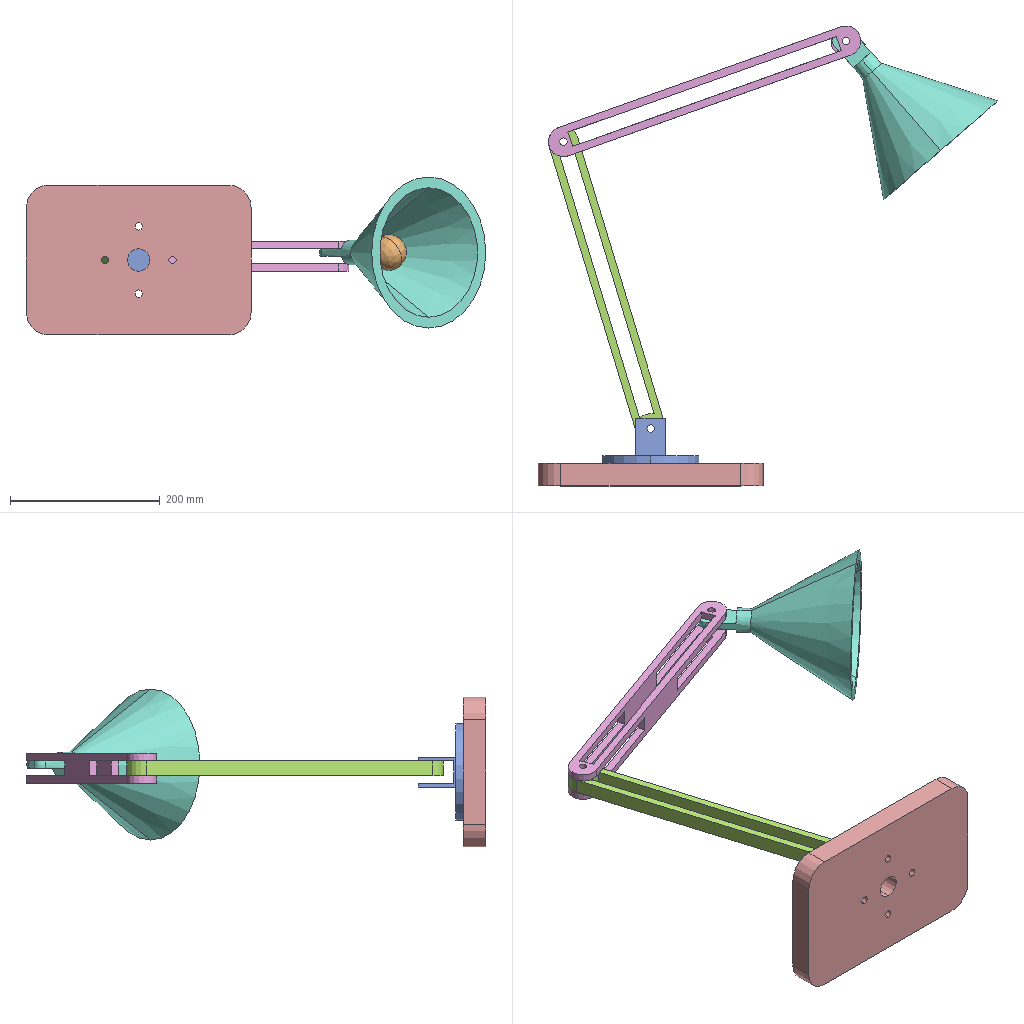Assembly | SolidWorks | 6 different items | 6 placed | box 613 x 613 x 211 mm
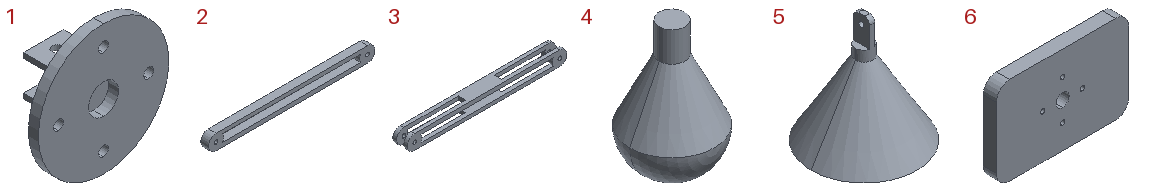Parts list (item | quantity | size | volume | features):
1 | x1 | 130 x 60 x 130 mm | 145337 mm3 | features ICE 4, Extrusion 1
2 | x1 | 440 x 20 x 40 mm | 197297 mm3 | features ICE 3, Extrusion 1
3 | x1 | 440 x 40 x 40 mm | 233504 mm3 | features ICE 4, MirrorPattern 2, Extrusion 1
4 | x1 | 47.821 x 47.821 x 75.022 mm | 59967 mm3 | features Revolution 1
5 | x1 | 201.428 x 201.428 x 209.626 mm | 565522 mm3 | features ICE 2, Fillet 1, RevCut 1, Revolution 1
6 | x1 | 300 x 30 x 200 mm | 1746192 mm3 | features Extrusion 1, Fillet 1, ICE 1
Mates (type | each side: item.copy, entity, surface, feature):
Concentric | 6.1 face cylinder Cut-Extrude1 | 1.1 face cylinder Cut-Extrude1 | 2 times
Coincident | 6.1 face plane Boss-Extrude1 | 1.1 face plane Boss-Extrude1
Concentric | 1.1 face cylinder Cut-Extrude3 | 2.1 face cylinder Cut-Extrude2
Coincident | 1.1 face plane Cut-Extrude2 | 2.1 face plane Boss-Extrude1
Concentric | 2.1 face cylinder Cut-Extrude2 | 3.1 face cylinder Cut-Extrude2
Coincident | 2.1 face plane Boss-Extrude1 | 3.1 face plane Boss-Extrude2
Concentric | 3.1 face cylinder Cut-Extrude2 | 5.1 face cylinder Cut-Extrude2
Coincident | 3.1 face plane Boss-Extrude2 | 5.1 face plane Cut-Extrude1
Concentric | 5.1 face cylinder Revolve1 | 4.1 face cylinder Revolve1
Coincident | 5.1 face plane Cut-Revolve1 | 4.1 face plane Revolve1